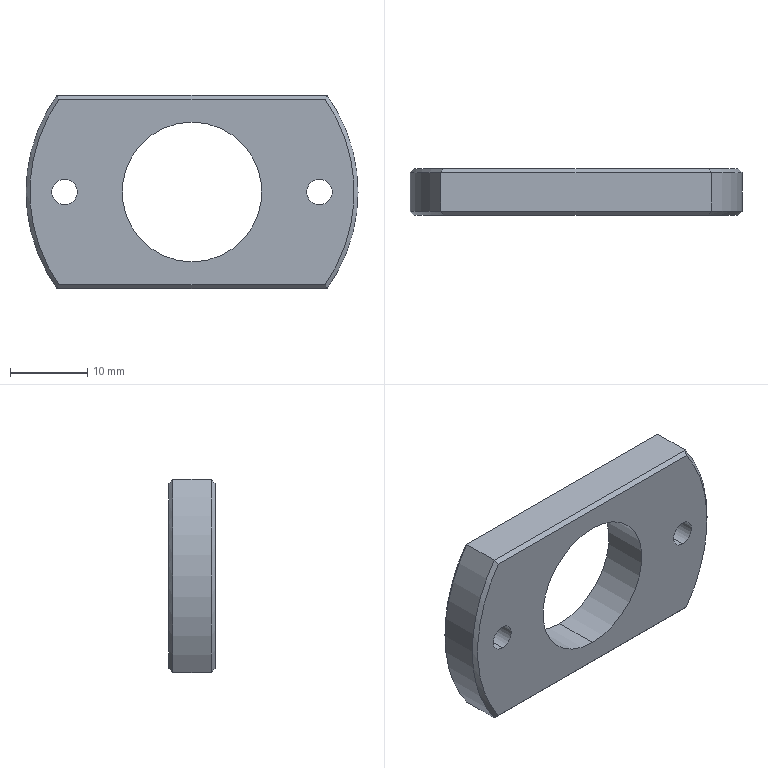Part | SolidWorks | features HoleWzd 2, Chamfer 1, Extrusion 1, ICE 1 | 1 solid | 20 faces | box 43 x 6 x 25 mm | volume 4389 mm3 | cylinder 8 | plane 8 | cone 4 | commonest cylinder face diameters 3.3 x4 18.1 x2 43 x2
STEP:
#1=CARTESIAN_POINT('',(0.,0.,-9.05));
#2=VERTEX_POINT('',#1);
#3=CARTESIAN_POINT('',(0.,0.,9.05));
#4=VERTEX_POINT('',#3);
#5=CARTESIAN_POINT('',(0.,0.,0.));
#6=DIRECTION('',(0.,1.,0.));
#7=DIRECTION('',(0.,0.,1.));
#8=AXIS2_PLACEMENT_3D('',#5,#6,#7);
#9=CIRCLE('',#8,9.05);
#10=EDGE_CURVE('',#2,#4,#9,.T.);
#11=ORIENTED_EDGE('',*,*,#10,.F.);
#12=CARTESIAN_POINT('',(0.,6.,-9.05));
#13=VERTEX_POINT('',#12);
#14=CARTESIAN_POINT('',(0.,6.,-9.05));
#15=DIRECTION('',(0.,1.,0.));
#16=VECTOR('',#15,1000.);
#17=LINE('',#14,#16);
#18=EDGE_CURVE('',#2,#13,#17,.T.);
#19=ORIENTED_EDGE('',*,*,#18,.T.);
#20=CARTESIAN_POINT('',(0.,6.,9.05));
#21=VERTEX_POINT('',#20);
#22=CARTESIAN_POINT('',(0.,6.,0.));
#23=DIRECTION('',(0.,1.,0.));
#24=DIRECTION('',(0.,0.,1.));
#25=AXIS2_PLACEMENT_3D('',#22,#23,#24);
#26=CIRCLE('',#25,9.05);
#27=EDGE_CURVE('',#13,#21,#26,.T.);
#28=ORIENTED_EDGE('',*,*,#27,.T.);
#29=CARTESIAN_POINT('',(0.,6.,9.05));
#30=DIRECTION('',(0.,1.,0.));
#31=VECTOR('',#30,1000.);
#32=LINE('',#29,#31);
#33=EDGE_CURVE('',#4,#21,#32,.T.);
#34=ORIENTED_EDGE('',*,*,#33,.F.);
#35=EDGE_LOOP('',(#11,#19,#28,#34));
#36=FACE_OUTER_BOUND('',#35,.T.);
#37=CARTESIAN_POINT('',(0.,6.,0.));
#38=DIRECTION('',(0.,1.,0.));
#39=DIRECTION('',(0.,0.,1.));
#40=AXIS2_PLACEMENT_3D('',#37,#38,#39);
#41=CYLINDRICAL_SURFACE('',#40,9.05);
#42=ADVANCED_FACE('',(#36),#41,.F.);
#43=CARTESIAN_POINT('',(-16.5,0.,-1.65));
#44=VERTEX_POINT('',#43);
#45=CARTESIAN_POINT('',(-16.5,0.,1.65));
#46=VERTEX_POINT('',#45);
#47=CARTESIAN_POINT('',(-16.5,0.,0.));
#48=DIRECTION('',(0.,1.,0.));
#49=DIRECTION('',(0.,0.,1.));
#50=AXIS2_PLACEMENT_3D('',#47,#48,#49);
#51=CIRCLE('',#50,1.65);
#52=EDGE_CURVE('',#44,#46,#51,.T.);
#53=ORIENTED_EDGE('',*,*,#52,.F.);
#54=CARTESIAN_POINT('',(-16.5,6.,-1.65));
#55=VERTEX_POINT('',#54);
#56=CARTESIAN_POINT('',(-16.5,6.,-1.65));
#57=DIRECTION('',(0.,1.,0.));
#58=VECTOR('',#57,1000.);
#59=LINE('',#56,#58);
#60=EDGE_CURVE('',#44,#55,#59,.T.);
#61=ORIENTED_EDGE('',*,*,#60,.T.);
#62=CARTESIAN_POINT('',(-16.5,6.,1.65));
#63=VERTEX_POINT('',#62);
#64=CARTESIAN_POINT('',(-16.5,6.,0.));
#65=DIRECTION('',(0.,1.,0.));
#66=DIRECTION('',(0.,0.,1.));
#67=AXIS2_PLACEMENT_3D('',#64,#65,#66);
#68=CIRCLE('',#67,1.65);
#69=EDGE_CURVE('',#55,#63,#68,.T.);
#70=ORIENTED_EDGE('',*,*,#69,.T.);
#71=CARTESIAN_POINT('',(-16.5,6.,1.65));
#72=DIRECTION('',(0.,1.,0.));
#73=VECTOR('',#72,1000.);
#74=LINE('',#71,#73);
#75=EDGE_CURVE('',#46,#63,#74,.T.);
#76=ORIENTED_EDGE('',*,*,#75,.F.);
#77=EDGE_LOOP('',(#53,#61,#70,#76));
#78=FACE_OUTER_BOUND('',#77,.T.);
#79=CARTESIAN_POINT('',(-16.5,6.,0.));
#80=DIRECTION('',(0.,1.,0.));
#81=DIRECTION('',(0.,0.,1.));
#82=AXIS2_PLACEMENT_3D('',#79,#80,#81);
#83=CYLINDRICAL_SURFACE('',#82,1.65);
#84=ADVANCED_FACE('',(#78),#83,.F.);
#85=CARTESIAN_POINT('',(16.5,0.,-1.65));
#86=VERTEX_POINT('',#85);
#87=CARTESIAN_POINT('',(16.5,0.,1.65));
#88=VERTEX_POINT('',#87);
#89=CARTESIAN_POINT('',(16.5,0.,0.));
#90=DIRECTION('',(0.,1.,0.));
#91=DIRECTION('',(0.,0.,1.));
#92=AXIS2_PLACEMENT_3D('',#89,#90,#91);
#93=CIRCLE('',#92,1.65);
#94=EDGE_CURVE('',#86,#88,#93,.T.);
#95=ORIENTED_EDGE('',*,*,#94,.F.);
#96=CARTESIAN_POINT('',(16.5,6.,-1.65));
#97=VERTEX_POINT('',#96);
#98=CARTESIAN_POINT('',(16.5,6.,-1.65));
#99=DIRECTION('',(0.,1.,0.));
#100=VECTOR('',#99,1000.);
#101=LINE('',#98,#100);
#102=EDGE_CURVE('',#86,#97,#101,.T.);
#103=ORIENTED_EDGE('',*,*,#102,.T.);
#104=CARTESIAN_POINT('',(16.5,6.,1.65));
#105=VERTEX_POINT('',#104);
#106=CARTESIAN_POINT('',(16.5,6.,0.));
#107=DIRECTION('',(0.,1.,0.));
#108=DIRECTION('',(0.,0.,1.));
#109=AXIS2_PLACEMENT_3D('',#106,#107,#108);
#110=CIRCLE('',#109,1.65);
#111=EDGE_CURVE('',#97,#105,#110,.T.);
#112=ORIENTED_EDGE('',*,*,#111,.T.);
#113=CARTESIAN_POINT('',(16.5,6.,1.65));
#114=DIRECTION('',(0.,1.,0.));
#115=VECTOR('',#114,1000.);
#116=LINE('',#113,#115);
#117=EDGE_CURVE('',#88,#105,#116,.T.);
#118=ORIENTED_EDGE('',*,*,#117,.F.);
#119=EDGE_LOOP('',(#95,#103,#112,#118));
#120=FACE_OUTER_BOUND('',#119,.T.);
#121=CARTESIAN_POINT('',(16.5,6.,0.));
#122=DIRECTION('',(0.,1.,0.));
#123=DIRECTION('',(0.,0.,1.));
#124=AXIS2_PLACEMENT_3D('',#121,#122,#123);
#125=CYLINDRICAL_SURFACE('',#124,1.65);
#126=ADVANCED_FACE('',(#120),#125,.F.);
#127=CARTESIAN_POINT('',(17.493,5.5,12.5));
#128=VERTEX_POINT('',#127);
#129=CARTESIAN_POINT('',(17.493,0.5,12.5));
#130=VERTEX_POINT('',#129);
#131=CARTESIAN_POINT('',(17.493,6.,12.5));
#132=DIRECTION('',(0.,-1.,0.));
#133=VECTOR('',#132,1000.);
#134=LINE('',#131,#133);
#135=EDGE_CURVE('',#128,#130,#134,.T.);
#136=ORIENTED_EDGE('',*,*,#135,.T.);
#137=CARTESIAN_POINT('',(17.493,0.5,-12.5));
#138=VERTEX_POINT('',#137);
#139=CARTESIAN_POINT('',(0.,0.5,0.));
#140=DIRECTION('',(0.,1.,0.));
#141=DIRECTION('',(0.,0.,1.));
#142=AXIS2_PLACEMENT_3D('',#139,#140,#141);
#143=CIRCLE('',#142,21.5);
#144=EDGE_CURVE('',#130,#138,#143,.T.);
#145=ORIENTED_EDGE('',*,*,#144,.T.);
#146=CARTESIAN_POINT('',(17.493,5.5,-12.5));
#147=VERTEX_POINT('',#146);
#148=CARTESIAN_POINT('',(17.493,6.,-12.5));
#149=DIRECTION('',(0.,1.,0.));
#150=VECTOR('',#149,1000.);
#151=LINE('',#148,#150);
#152=EDGE_CURVE('',#138,#147,#151,.T.);
#153=ORIENTED_EDGE('',*,*,#152,.T.);
#154=CARTESIAN_POINT('',(0.,5.5,0.));
#155=DIRECTION('',(0.,-1.,0.));
#156=DIRECTION('',(0.,0.,1.));
#157=AXIS2_PLACEMENT_3D('',#154,#155,#156);
#158=CIRCLE('',#157,21.5);
#159=EDGE_CURVE('',#147,#128,#158,.T.);
#160=ORIENTED_EDGE('',*,*,#159,.T.);
#161=EDGE_LOOP('',(#136,#145,#153,#160));
#162=FACE_OUTER_BOUND('',#161,.T.);
#163=CARTESIAN_POINT('',(0.,6.,0.));
#164=DIRECTION('',(0.,-1.,0.));
#165=DIRECTION('',(0.,0.,-1.));
#166=AXIS2_PLACEMENT_3D('',#163,#164,#165);
#167=CYLINDRICAL_SURFACE('',#166,21.5);
#168=ADVANCED_FACE('',(#162),#167,.T.);
#169=CARTESIAN_POINT('',(-17.493,5.5,-12.5));
#170=VERTEX_POINT('',#169);
#171=CARTESIAN_POINT('',(-17.493,0.5,-12.5));
#172=VERTEX_POINT('',#171);
#173=CARTESIAN_POINT('',(-17.493,6.,-12.5));
#174=DIRECTION('',(0.,-1.,0.));
#175=VECTOR('',#174,1000.);
#176=LINE('',#173,#175);
#177=EDGE_CURVE('',#170,#172,#176,.T.);
#178=ORIENTED_EDGE('',*,*,#177,.T.);
#179=CARTESIAN_POINT('',(-17.493,0.5,12.5));
#180=VERTEX_POINT('',#179);
#181=CARTESIAN_POINT('',(0.,0.5,0.));
#182=DIRECTION('',(0.,1.,0.));
#183=DIRECTION('',(0.,0.,1.));
#184=AXIS2_PLACEMENT_3D('',#181,#182,#183);
#185=CIRCLE('',#184,21.5);
#186=EDGE_CURVE('',#172,#180,#185,.T.);
#187=ORIENTED_EDGE('',*,*,#186,.T.);
#188=CARTESIAN_POINT('',(-17.493,5.5,12.5));
#189=VERTEX_POINT('',#188);
#190=CARTESIAN_POINT('',(-17.493,6.,12.5));
#191=DIRECTION('',(0.,1.,0.));
#192=VECTOR('',#191,1000.);
#193=LINE('',#190,#192);
#194=EDGE_CURVE('',#180,#189,#193,.T.);
#195=ORIENTED_EDGE('',*,*,#194,.T.);
#196=CARTESIAN_POINT('',(0.,5.5,0.));
#197=DIRECTION('',(0.,-1.,0.));
#198=DIRECTION('',(0.,0.,1.));
#199=AXIS2_PLACEMENT_3D('',#196,#197,#198);
#200=CIRCLE('',#199,21.5);
#201=EDGE_CURVE('',#189,#170,#200,.T.);
#202=ORIENTED_EDGE('',*,*,#201,.T.);
#203=EDGE_LOOP('',(#178,#187,#195,#202));
#204=FACE_OUTER_BOUND('',#203,.T.);
#205=CARTESIAN_POINT('',(0.,6.,0.));
#206=DIRECTION('',(0.,-1.,0.));
#207=DIRECTION('',(0.,0.,-1.));
#208=AXIS2_PLACEMENT_3D('',#205,#206,#207);
#209=CYLINDRICAL_SURFACE('',#208,21.5);
#210=ADVANCED_FACE('',(#204),#209,.T.);
#211=CARTESIAN_POINT('',(-17.234,6.,12.));
#212=VERTEX_POINT('',#211);
#213=CARTESIAN_POINT('',(17.234,6.,12.));
#214=VERTEX_POINT('',#213);
#215=CARTESIAN_POINT('',(17.493,6.,12.));
#216=DIRECTION('',(1.,0.,0.));
#217=VECTOR('',#216,1000.);
#218=LINE('',#215,#217);
#219=EDGE_CURVE('',#212,#214,#218,.T.);
#220=ORIENTED_EDGE('',*,*,#219,.T.);
#221=CARTESIAN_POINT('',(17.234,6.,-12.));
#222=VERTEX_POINT('',#221);
#223=CARTESIAN_POINT('',(0.,6.,0.));
#224=DIRECTION('',(0.,1.,0.));
#225=DIRECTION('',(0.,0.,1.));
#226=AXIS2_PLACEMENT_3D('',#223,#224,#225);
#227=CIRCLE('',#226,21.);
#228=EDGE_CURVE('',#214,#222,#227,.T.);
#229=ORIENTED_EDGE('',*,*,#228,.T.);
#230=CARTESIAN_POINT('',(-17.234,6.,-12.));
#231=VERTEX_POINT('',#230);
#232=CARTESIAN_POINT('',(-17.493,6.,-12.));
#233=DIRECTION('',(-1.,0.,0.));
#234=VECTOR('',#233,1000.);
#235=LINE('',#232,#234);
#236=EDGE_CURVE('',#222,#231,#235,.T.);
#237=ORIENTED_EDGE('',*,*,#236,.T.);
#238=CARTESIAN_POINT('',(0.,6.,0.));
#239=DIRECTION('',(0.,1.,0.));
#240=DIRECTION('',(0.,0.,1.));
#241=AXIS2_PLACEMENT_3D('',#238,#239,#240);
#242=CIRCLE('',#241,21.);
#243=EDGE_CURVE('',#231,#212,#242,.T.);
#244=ORIENTED_EDGE('',*,*,#243,.T.);
#245=EDGE_LOOP('',(#220,#229,#237,#244));
#246=FACE_OUTER_BOUND('',#245,.T.);
#247=CARTESIAN_POINT('',(0.,6.,0.));
#248=DIRECTION('',(0.,1.,0.));
#249=DIRECTION('',(0.,0.,1.));
#250=AXIS2_PLACEMENT_3D('',#247,#248,#249);
#251=CIRCLE('',#250,9.05);
#252=EDGE_CURVE('',#21,#13,#251,.T.);
#253=ORIENTED_EDGE('',*,*,#252,.F.);
#254=ORIENTED_EDGE('',*,*,#27,.F.);
#255=EDGE_LOOP('',(#253,#254));
#256=FACE_BOUND('',#255,.T.);
#257=CARTESIAN_POINT('',(-16.5,6.,0.));
#258=DIRECTION('',(0.,1.,0.));
#259=DIRECTION('',(0.,0.,1.));
#260=AXIS2_PLACEMENT_3D('',#257,#258,#259);
#261=CIRCLE('',#260,1.65);
#262=EDGE_CURVE('',#63,#55,#261,.T.);
#263=ORIENTED_EDGE('',*,*,#262,.F.);
#264=ORIENTED_EDGE('',*,*,#69,.F.);
#265=EDGE_LOOP('',(#263,#264));
#266=FACE_BOUND('',#265,.T.);
#267=CARTESIAN_POINT('',(16.5,6.,0.));
#268=DIRECTION('',(0.,1.,0.));
#269=DIRECTION('',(0.,0.,1.));
#270=AXIS2_PLACEMENT_3D('',#267,#268,#269);
#271=CIRCLE('',#270,1.65);
#272=EDGE_CURVE('',#105,#97,#271,.T.);
#273=ORIENTED_EDGE('',*,*,#272,.F.);
#274=ORIENTED_EDGE('',*,*,#111,.F.);
#275=EDGE_LOOP('',(#273,#274));
#276=FACE_BOUND('',#275,.T.);
#277=CARTESIAN_POINT('',(0.,6.,0.));
#278=DIRECTION('',(0.,1.,0.));
#279=DIRECTION('',(0.,0.,1.));
#280=AXIS2_PLACEMENT_3D('',#277,#278,#279);
#281=PLANE('',#280);
#282=ADVANCED_FACE('',(#246,#256,#266,#276),#281,.T.);
#283=CARTESIAN_POINT('',(17.234,0.,12.));
#284=VERTEX_POINT('',#283);
#285=CARTESIAN_POINT('',(-17.234,0.,12.));
#286=VERTEX_POINT('',#285);
#287=CARTESIAN_POINT('',(0.,0.,12.));
#288=DIRECTION('',(-1.,0.,0.));
#289=VECTOR('',#288,1000.);
#290=LINE('',#287,#289);
#291=EDGE_CURVE('',#284,#286,#290,.T.);
#292=ORIENTED_EDGE('',*,*,#291,.T.);
#293=CARTESIAN_POINT('',(-17.234,0.,-12.));
#294=VERTEX_POINT('',#293);
#295=CARTESIAN_POINT('',(0.,0.,0.));
#296=DIRECTION('',(0.,-1.,0.));
#297=DIRECTION('',(0.,0.,1.));
#298=AXIS2_PLACEMENT_3D('',#295,#296,#297);
#299=CIRCLE('',#298,21.);
#300=EDGE_CURVE('',#286,#294,#299,.T.);
#301=ORIENTED_EDGE('',*,*,#300,.T.);
#302=CARTESIAN_POINT('',(17.234,0.,-12.));
#303=VERTEX_POINT('',#302);
#304=CARTESIAN_POINT('',(0.,0.,-12.));
#305=DIRECTION('',(1.,0.,0.));
#306=VECTOR('',#305,1000.);
#307=LINE('',#304,#306);
#308=EDGE_CURVE('',#294,#303,#307,.T.);
#309=ORIENTED_EDGE('',*,*,#308,.T.);
#310=CARTESIAN_POINT('',(0.,0.,0.));
#311=DIRECTION('',(0.,-1.,0.));
#312=DIRECTION('',(0.,0.,1.));
#313=AXIS2_PLACEMENT_3D('',#310,#311,#312);
#314=CIRCLE('',#313,21.);
#315=EDGE_CURVE('',#303,#284,#314,.T.);
#316=ORIENTED_EDGE('',*,*,#315,.T.);
#317=EDGE_LOOP('',(#292,#301,#309,#316));
#318=FACE_OUTER_BOUND('',#317,.T.);
#319=CARTESIAN_POINT('',(0.,0.,0.));
#320=DIRECTION('',(0.,1.,0.));
#321=DIRECTION('',(0.,0.,1.));
#322=AXIS2_PLACEMENT_3D('',#319,#320,#321);
#323=CIRCLE('',#322,9.05);
#324=EDGE_CURVE('',#4,#2,#323,.T.);
#325=ORIENTED_EDGE('',*,*,#324,.T.);
#326=ORIENTED_EDGE('',*,*,#10,.T.);
#327=EDGE_LOOP('',(#325,#326));
#328=FACE_BOUND('',#327,.T.);
#329=CARTESIAN_POINT('',(-16.5,0.,0.));
#330=DIRECTION('',(0.,1.,0.));
#331=DIRECTION('',(0.,0.,1.));
#332=AXIS2_PLACEMENT_3D('',#329,#330,#331);
#333=CIRCLE('',#332,1.65);
#334=EDGE_CURVE('',#46,#44,#333,.T.);
#335=ORIENTED_EDGE('',*,*,#334,.T.);
#336=ORIENTED_EDGE('',*,*,#52,.T.);
#337=EDGE_LOOP('',(#335,#336));
#338=FACE_BOUND('',#337,.T.);
#339=CARTESIAN_POINT('',(16.5,0.,0.));
#340=DIRECTION('',(0.,1.,0.));
#341=DIRECTION('',(0.,0.,1.));
#342=AXIS2_PLACEMENT_3D('',#339,#340,#341);
#343=CIRCLE('',#342,1.65);
#344=EDGE_CURVE('',#88,#86,#343,.T.);
#345=ORIENTED_EDGE('',*,*,#344,.T.);
#346=ORIENTED_EDGE('',*,*,#94,.T.);
#347=EDGE_LOOP('',(#345,#346));
#348=FACE_BOUND('',#347,.T.);
#349=CARTESIAN_POINT('',(0.,0.,0.));
#350=DIRECTION('',(0.,1.,0.));
#351=DIRECTION('',(0.,0.,1.));
#352=AXIS2_PLACEMENT_3D('',#349,#350,#351);
#353=PLANE('',#352);
#354=ADVANCED_FACE('',(#318,#328,#338,#348),#353,.F.);
#355=ORIENTED_EDGE('',*,*,#102,.F.);
#356=ORIENTED_EDGE('',*,*,#344,.F.);
#357=ORIENTED_EDGE('',*,*,#117,.T.);
#358=ORIENTED_EDGE('',*,*,#272,.T.);
#359=EDGE_LOOP('',(#355,#356,#357,#358));
#360=FACE_OUTER_BOUND('',#359,.T.);
#361=CARTESIAN_POINT('',(16.5,6.,0.));
#362=DIRECTION('',(0.,1.,0.));
#363=DIRECTION('',(0.,0.,1.));
#364=AXIS2_PLACEMENT_3D('',#361,#362,#363);
#365=CYLINDRICAL_SURFACE('',#364,1.65);
#366=ADVANCED_FACE('',(#360),#365,.F.);
#367=ORIENTED_EDGE('',*,*,#60,.F.);
#368=ORIENTED_EDGE('',*,*,#334,.F.);
#369=ORIENTED_EDGE('',*,*,#75,.T.);
#370=ORIENTED_EDGE('',*,*,#262,.T.);
#371=EDGE_LOOP('',(#367,#368,#369,#370));
#372=FACE_OUTER_BOUND('',#371,.T.);
#373=CARTESIAN_POINT('',(-16.5,6.,0.));
#374=DIRECTION('',(0.,1.,0.));
#375=DIRECTION('',(0.,0.,1.));
#376=AXIS2_PLACEMENT_3D('',#373,#374,#375);
#377=CYLINDRICAL_SURFACE('',#376,1.65);
#378=ADVANCED_FACE('',(#372),#377,.F.);
#379=ORIENTED_EDGE('',*,*,#152,.F.);
#380=CARTESIAN_POINT('',(-45.306,0.5,-12.5));
#381=DIRECTION('',(-1.,0.,0.));
#382=VECTOR('',#381,1000.);
#383=LINE('',#380,#382);
#384=EDGE_CURVE('',#138,#172,#383,.T.);
#385=ORIENTED_EDGE('',*,*,#384,.T.);
#386=ORIENTED_EDGE('',*,*,#177,.F.);
#387=CARTESIAN_POINT('',(17.493,5.5,-12.5));
#388=DIRECTION('',(1.,0.,0.));
#389=VECTOR('',#388,1000.);
#390=LINE('',#387,#389);
#391=EDGE_CURVE('',#170,#147,#390,.T.);
#392=ORIENTED_EDGE('',*,*,#391,.T.);
#393=EDGE_LOOP('',(#379,#385,#386,#392));
#394=FACE_OUTER_BOUND('',#393,.T.);
#395=CARTESIAN_POINT('',(-45.306,0.,-12.5));
#396=DIRECTION('',(0.,0.,1.));
#397=DIRECTION('',(1.,0.,0.));
#398=AXIS2_PLACEMENT_3D('',#395,#396,#397);
#399=PLANE('',#398);
#400=ADVANCED_FACE('',(#394),#399,.F.);
#401=ORIENTED_EDGE('',*,*,#194,.F.);
#402=CARTESIAN_POINT('',(94.721,0.5,12.5));
#403=DIRECTION('',(1.,0.,0.));
#404=VECTOR('',#403,1000.);
#405=LINE('',#402,#404);
#406=EDGE_CURVE('',#180,#130,#405,.T.);
#407=ORIENTED_EDGE('',*,*,#406,.T.);
#408=ORIENTED_EDGE('',*,*,#135,.F.);
#409=CARTESIAN_POINT('',(-17.493,5.5,12.5));
#410=DIRECTION('',(-1.,0.,0.));
#411=VECTOR('',#410,1000.);
#412=LINE('',#409,#411);
#413=EDGE_CURVE('',#128,#189,#412,.T.);
#414=ORIENTED_EDGE('',*,*,#413,.T.);
#415=EDGE_LOOP('',(#401,#407,#408,#414));
#416=FACE_OUTER_BOUND('',#415,.T.);
#417=CARTESIAN_POINT('',(94.721,0.,12.5));
#418=DIRECTION('',(0.,0.,-1.));
#419=DIRECTION('',(-1.,0.,0.));
#420=AXIS2_PLACEMENT_3D('',#417,#418,#419);
#421=PLANE('',#420);
#422=ADVANCED_FACE('',(#416),#421,.F.);
#423=ORIENTED_EDGE('',*,*,#18,.F.);
#424=ORIENTED_EDGE('',*,*,#324,.F.);
#425=ORIENTED_EDGE('',*,*,#33,.T.);
#426=ORIENTED_EDGE('',*,*,#252,.T.);
#427=EDGE_LOOP('',(#423,#424,#425,#426));
#428=FACE_OUTER_BOUND('',#427,.T.);
#429=CARTESIAN_POINT('',(0.,6.,0.));
#430=DIRECTION('',(0.,1.,0.));
#431=DIRECTION('',(0.,0.,1.));
#432=AXIS2_PLACEMENT_3D('',#429,#430,#431);
#433=CYLINDRICAL_SURFACE('',#432,9.05);
#434=ADVANCED_FACE('',(#428),#433,.F.);
#435=CARTESIAN_POINT('',(17.234,0.,12.));
#436=CARTESIAN_POINT('',(17.321,0.1665,12.167));
#437=CARTESIAN_POINT('',(17.407,0.3332,12.333));
#438=CARTESIAN_POINT('',(17.493,0.5,12.5));
#439=B_SPLINE_CURVE_WITH_KNOTS('',3,(#435,#436,#437,#438),.UNSPECIFIED.,.F.,.F.,(4,4),(0.,0.0007531),.UNSPECIFIED.);
#440=EDGE_CURVE('',#284,#130,#439,.T.);
#441=ORIENTED_EDGE('',*,*,#440,.F.);
#442=ORIENTED_EDGE('',*,*,#315,.F.);
#443=CARTESIAN_POINT('',(17.493,0.5,-12.5));
#444=CARTESIAN_POINT('',(17.407,0.3332,-12.333));
#445=CARTESIAN_POINT('',(17.321,0.1665,-12.167));
#446=CARTESIAN_POINT('',(17.234,0.,-12.));
#447=B_SPLINE_CURVE_WITH_KNOTS('',3,(#443,#444,#445,#446),.UNSPECIFIED.,.F.,.F.,(4,4),(0.,0.0007531),.UNSPECIFIED.);
#448=EDGE_CURVE('',#138,#303,#447,.T.);
#449=ORIENTED_EDGE('',*,*,#448,.F.);
#450=ORIENTED_EDGE('',*,*,#144,.F.);
#451=EDGE_LOOP('',(#441,#442,#449,#450));
#452=FACE_OUTER_BOUND('',#451,.T.);
#453=CARTESIAN_POINT('',(0.,0.5,0.));
#454=DIRECTION('',(0.,1.,0.));
#455=DIRECTION('',(0.,0.,1.));
#456=AXIS2_PLACEMENT_3D('',#453,#454,#455);
#457=CONICAL_SURFACE('',#456,21.5,0.7854);
#458=ADVANCED_FACE('',(#452),#457,.T.);
#459=ORIENTED_EDGE('',*,*,#448,.T.);
#460=ORIENTED_EDGE('',*,*,#308,.F.);
#461=CARTESIAN_POINT('',(-17.493,0.5,-12.5));
#462=CARTESIAN_POINT('',(-17.407,0.3332,-12.333));
#463=CARTESIAN_POINT('',(-17.321,0.1665,-12.167));
#464=CARTESIAN_POINT('',(-17.234,0.,-12.));
#465=B_SPLINE_CURVE_WITH_KNOTS('',3,(#461,#462,#463,#464),.UNSPECIFIED.,.F.,.F.,(4,4),(0.,0.0007531),.UNSPECIFIED.);
#466=EDGE_CURVE('',#172,#294,#465,.T.);
#467=ORIENTED_EDGE('',*,*,#466,.F.);
#468=ORIENTED_EDGE('',*,*,#384,.F.);
#469=EDGE_LOOP('',(#459,#460,#467,#468));
#470=FACE_OUTER_BOUND('',#469,.T.);
#471=CARTESIAN_POINT('',(0.,0.,-12.));
#472=DIRECTION('',(0.,0.7071,0.7071));
#473=DIRECTION('',(1.,0.,0.));
#474=AXIS2_PLACEMENT_3D('',#471,#472,#473);
#475=PLANE('',#474);
#476=ADVANCED_FACE('',(#470),#475,.F.);
#477=ORIENTED_EDGE('',*,*,#440,.T.);
#478=ORIENTED_EDGE('',*,*,#406,.F.);
#479=CARTESIAN_POINT('',(-17.234,0.,12.));
#480=CARTESIAN_POINT('',(-17.321,0.1665,12.167));
#481=CARTESIAN_POINT('',(-17.407,0.3332,12.333));
#482=CARTESIAN_POINT('',(-17.493,0.5,12.5));
#483=B_SPLINE_CURVE_WITH_KNOTS('',3,(#479,#480,#481,#482),.UNSPECIFIED.,.F.,.F.,(4,4),(0.,0.0007531),.UNSPECIFIED.);
#484=EDGE_CURVE('',#286,#180,#483,.T.);
#485=ORIENTED_EDGE('',*,*,#484,.F.);
#486=ORIENTED_EDGE('',*,*,#291,.F.);
#487=EDGE_LOOP('',(#477,#478,#485,#486));
#488=FACE_OUTER_BOUND('',#487,.T.);
#489=CARTESIAN_POINT('',(0.,0.,12.));
#490=DIRECTION('',(0.,0.7071,-0.7071));
#491=DIRECTION('',(-1.,0.,0.));
#492=AXIS2_PLACEMENT_3D('',#489,#490,#491);
#493=PLANE('',#492);
#494=ADVANCED_FACE('',(#488),#493,.F.);
#495=ORIENTED_EDGE('',*,*,#466,.T.);
#496=ORIENTED_EDGE('',*,*,#300,.F.);
#497=ORIENTED_EDGE('',*,*,#484,.T.);
#498=ORIENTED_EDGE('',*,*,#186,.F.);
#499=EDGE_LOOP('',(#495,#496,#497,#498));
#500=FACE_OUTER_BOUND('',#499,.T.);
#501=CARTESIAN_POINT('',(0.,0.5,0.));
#502=DIRECTION('',(0.,1.,0.));
#503=DIRECTION('',(0.,0.,1.));
#504=AXIS2_PLACEMENT_3D('',#501,#502,#503);
#505=CONICAL_SURFACE('',#504,21.5,0.7854);
#506=ADVANCED_FACE('',(#500),#505,.T.);
#507=CARTESIAN_POINT('',(-17.493,5.5,-12.5));
#508=CARTESIAN_POINT('',(-17.407,5.667,-12.333));
#509=CARTESIAN_POINT('',(-17.321,5.833,-12.167));
#510=CARTESIAN_POINT('',(-17.234,6.,-12.));
#511=B_SPLINE_CURVE_WITH_KNOTS('',3,(#507,#508,#509,#510),.UNSPECIFIED.,.F.,.F.,(4,4),(0.,0.0007531),.UNSPECIFIED.);
#512=EDGE_CURVE('',#170,#231,#511,.T.);
#513=ORIENTED_EDGE('',*,*,#512,.F.);
#514=ORIENTED_EDGE('',*,*,#201,.F.);
#515=CARTESIAN_POINT('',(-17.234,6.,12.));
#516=CARTESIAN_POINT('',(-17.321,5.833,12.167));
#517=CARTESIAN_POINT('',(-17.407,5.667,12.333));
#518=CARTESIAN_POINT('',(-17.493,5.5,12.5));
#519=B_SPLINE_CURVE_WITH_KNOTS('',3,(#515,#516,#517,#518),.UNSPECIFIED.,.F.,.F.,(4,4),(0.,0.0007531),.UNSPECIFIED.);
#520=EDGE_CURVE('',#212,#189,#519,.T.);
#521=ORIENTED_EDGE('',*,*,#520,.F.);
#522=ORIENTED_EDGE('',*,*,#243,.F.);
#523=EDGE_LOOP('',(#513,#514,#521,#522));
#524=FACE_OUTER_BOUND('',#523,.T.);
#525=CARTESIAN_POINT('',(0.,6.,0.));
#526=DIRECTION('',(0.,-1.,0.));
#527=DIRECTION('',(0.,0.,-1.));
#528=AXIS2_PLACEMENT_3D('',#525,#526,#527);
#529=CONICAL_SURFACE('',#528,21.,0.7854);
#530=ADVANCED_FACE('',(#524),#529,.T.);
#531=ORIENTED_EDGE('',*,*,#520,.T.);
#532=ORIENTED_EDGE('',*,*,#413,.F.);
#533=CARTESIAN_POINT('',(17.234,6.,12.));
#534=CARTESIAN_POINT('',(17.321,5.833,12.167));
#535=CARTESIAN_POINT('',(17.407,5.667,12.333));
#536=CARTESIAN_POINT('',(17.493,5.5,12.5));
#537=B_SPLINE_CURVE_WITH_KNOTS('',3,(#533,#534,#535,#536),.UNSPECIFIED.,.F.,.F.,(4,4),(0.,0.0007531),.UNSPECIFIED.);
#538=EDGE_CURVE('',#214,#128,#537,.T.);
#539=ORIENTED_EDGE('',*,*,#538,.F.);
#540=ORIENTED_EDGE('',*,*,#219,.F.);
#541=EDGE_LOOP('',(#531,#532,#539,#540));
#542=FACE_OUTER_BOUND('',#541,.T.);
#543=CARTESIAN_POINT('',(94.721,5.5,12.5));
#544=DIRECTION('',(0.,0.7071,0.7071));
#545=DIRECTION('',(1.,0.,0.));
#546=AXIS2_PLACEMENT_3D('',#543,#544,#545);
#547=PLANE('',#546);
#548=ADVANCED_FACE('',(#542),#547,.T.);
#549=ORIENTED_EDGE('',*,*,#512,.T.);
#550=ORIENTED_EDGE('',*,*,#236,.F.);
#551=CARTESIAN_POINT('',(17.493,5.5,-12.5));
#552=CARTESIAN_POINT('',(17.407,5.667,-12.333));
#553=CARTESIAN_POINT('',(17.321,5.833,-12.167));
#554=CARTESIAN_POINT('',(17.234,6.,-12.));
#555=B_SPLINE_CURVE_WITH_KNOTS('',3,(#551,#552,#553,#554),.UNSPECIFIED.,.F.,.F.,(4,4),(0.,0.0007531),.UNSPECIFIED.);
#556=EDGE_CURVE('',#147,#222,#555,.T.);
#557=ORIENTED_EDGE('',*,*,#556,.F.);
#558=ORIENTED_EDGE('',*,*,#391,.F.);
#559=EDGE_LOOP('',(#549,#550,#557,#558));
#560=FACE_OUTER_BOUND('',#559,.T.);
#561=CARTESIAN_POINT('',(-45.306,5.5,-12.5));
#562=DIRECTION('',(0.,0.7071,-0.7071));
#563=DIRECTION('',(-1.,0.,0.));
#564=AXIS2_PLACEMENT_3D('',#561,#562,#563);
#565=PLANE('',#564);
#566=ADVANCED_FACE('',(#560),#565,.T.);
#567=ORIENTED_EDGE('',*,*,#538,.T.);
#568=ORIENTED_EDGE('',*,*,#159,.F.);
#569=ORIENTED_EDGE('',*,*,#556,.T.);
#570=ORIENTED_EDGE('',*,*,#228,.F.);
#571=EDGE_LOOP('',(#567,#568,#569,#570));
#572=FACE_OUTER_BOUND('',#571,.T.);
#573=CARTESIAN_POINT('',(0.,6.,0.));
#574=DIRECTION('',(0.,-1.,0.));
#575=DIRECTION('',(0.,0.,-1.));
#576=AXIS2_PLACEMENT_3D('',#573,#574,#575);
#577=CONICAL_SURFACE('',#576,21.,0.7854);
#578=ADVANCED_FACE('',(#572),#577,.T.);
#579=CLOSED_SHELL('',(#42,#84,#126,#168,#210,#282,#354,#366,#378,#400,#422,#434,#458,#476,#494,#506,#530,#548,#566,#578));
#580=MANIFOLD_SOLID_BREP('',#579);
#581=CARTESIAN_POINT('',(0.,0.,0.));
#582=DIRECTION('',(0.,0.,1.));
#583=DIRECTION('',(1.,0.,0.));
#584=AXIS2_PLACEMENT_3D('',#581,#582,#583);
#585=(LENGTH_UNIT()NAMED_UNIT(*)SI_UNIT(.MILLI.,.METRE.));
#586=UNCERTAINTY_MEASURE_WITH_UNIT(LENGTH_MEASURE(0.00001),#585,'','');
#587=(NAMED_UNIT(*)PLANE_ANGLE_UNIT()SI_UNIT($,.RADIAN.));
#588=(NAMED_UNIT(*)SI_UNIT($,.STERADIAN.)SOLID_ANGLE_UNIT());
#589=(GEOMETRIC_REPRESENTATION_CONTEXT(3)GLOBAL_UNCERTAINTY_ASSIGNED_CONTEXT((#586))GLOBAL_UNIT_ASSIGNED_CONTEXT((#585,#587,#588))REPRESENTATION_CONTEXT('',''));
#590=ADVANCED_BREP_SHAPE_REPRESENTATION('',(#580,#584),#589);